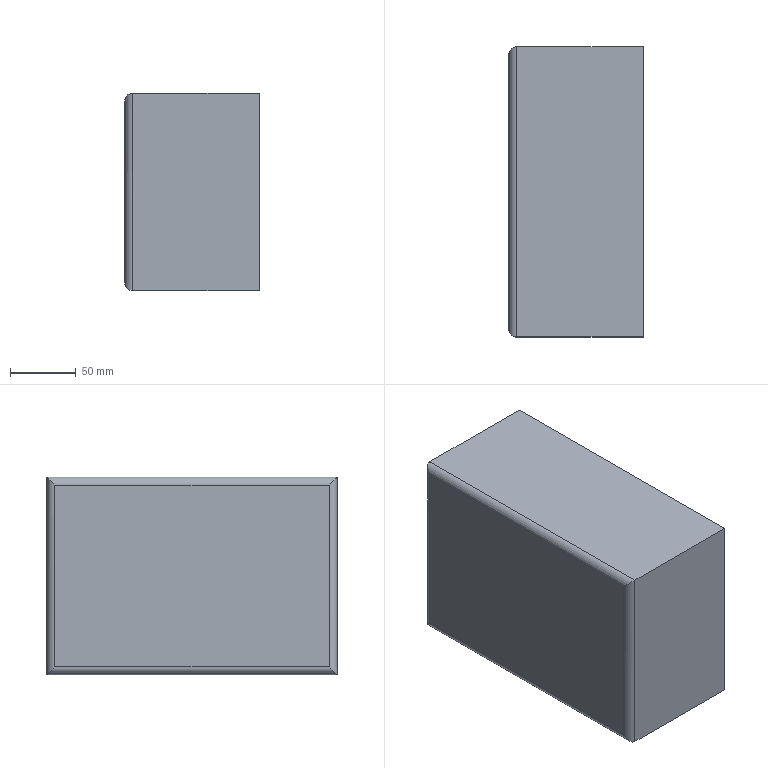Part | NX | 1 solid | 10 faces | box 102 x 220.092 x 150 mm | volume 3361772 mm3 | plane 6 | cylinder 4 | commonest cylinder face diameters 12 x4
STEP:
#1=CARTESIAN_POINT('',(-151.326,-99.951,581.553));
#2=VERTEX_POINT('',#1);
#3=CARTESIAN_POINT('',(-55.326,-99.951,581.553));
#4=VERTEX_POINT('',#3);
#5=CARTESIAN_POINT('',(-157.326,-99.951,581.553));
#6=DIRECTION('',(1.,0.,0.));
#7=VECTOR('',#6,1.);
#8=LINE('',#5,#7);
#9=EDGE_CURVE('',#2,#4,#8,.T.);
#10=ORIENTED_EDGE('',*,*,#9,.F.);
#11=CARTESIAN_POINT('',(-151.326,120.141,581.553));
#12=VERTEX_POINT('',#11);
#13=CARTESIAN_POINT('',(-151.326,120.141,581.553));
#14=DIRECTION('',(0.,1.,0.));
#15=VECTOR('',#14,1.);
#16=LINE('',#13,#15);
#17=EDGE_CURVE('',#2,#12,#16,.T.);
#18=ORIENTED_EDGE('',*,*,#17,.T.);
#19=CARTESIAN_POINT('',(-55.326,120.141,581.553));
#20=VERTEX_POINT('',#19);
#21=CARTESIAN_POINT('',(-157.326,120.141,581.553));
#22=DIRECTION('',(1.,0.,0.));
#23=VECTOR('',#22,1.);
#24=LINE('',#21,#23);
#25=EDGE_CURVE('',#12,#20,#24,.T.);
#26=ORIENTED_EDGE('',*,*,#25,.T.);
#27=CARTESIAN_POINT('',(-55.326,120.141,581.553));
#28=DIRECTION('',(0.,-1.,0.));
#29=VECTOR('',#28,1.);
#30=LINE('',#27,#29);
#31=EDGE_CURVE('',#20,#4,#30,.T.);
#32=ORIENTED_EDGE('',*,*,#31,.T.);
#33=EDGE_LOOP('',(#10,#18,#26,#32));
#34=FACE_OUTER_BOUND('',#33,.T.);
#35=CARTESIAN_POINT('',(-157.326,120.141,581.553));
#36=DIRECTION('',(0.,0.,1.));
#37=DIRECTION('',(1.,0.,0.));
#38=AXIS2_PLACEMENT_3D('',#35,#36,#37);
#39=PLANE('',#38);
#40=ADVANCED_FACE('',(#34),#39,.F.);
#41=CARTESIAN_POINT('',(-151.326,-99.951,731.553));
#42=VERTEX_POINT('',#41);
#43=CARTESIAN_POINT('',(-55.326,-99.951,731.553));
#44=VERTEX_POINT('',#43);
#45=CARTESIAN_POINT('',(-157.326,-99.951,731.553));
#46=DIRECTION('',(1.,0.,0.));
#47=VECTOR('',#46,1.);
#48=LINE('',#45,#47);
#49=EDGE_CURVE('',#42,#44,#48,.T.);
#50=ORIENTED_EDGE('',*,*,#49,.F.);
#51=CARTESIAN_POINT('',(-151.326,-99.951,581.553));
#52=DIRECTION('',(0.,0.,-1.));
#53=VECTOR('',#52,1.);
#54=LINE('',#51,#53);
#55=EDGE_CURVE('',#42,#2,#54,.T.);
#56=ORIENTED_EDGE('',*,*,#55,.T.);
#57=ORIENTED_EDGE('',*,*,#9,.T.);
#58=CARTESIAN_POINT('',(-55.326,-99.951,581.553));
#59=DIRECTION('',(0.,0.,1.));
#60=VECTOR('',#59,1.);
#61=LINE('',#58,#60);
#62=EDGE_CURVE('',#4,#44,#61,.T.);
#63=ORIENTED_EDGE('',*,*,#62,.T.);
#64=EDGE_LOOP('',(#50,#56,#57,#63));
#65=FACE_OUTER_BOUND('',#64,.T.);
#66=CARTESIAN_POINT('',(-157.326,-99.951,581.553));
#67=DIRECTION('',(0.,1.,0.));
#68=DIRECTION('',(0.,0.,1.));
#69=AXIS2_PLACEMENT_3D('',#66,#67,#68);
#70=PLANE('',#69);
#71=ADVANCED_FACE('',(#65),#70,.F.);
#72=CARTESIAN_POINT('',(-151.326,120.141,731.553));
#73=VERTEX_POINT('',#72);
#74=CARTESIAN_POINT('',(-55.326,120.141,731.553));
#75=VERTEX_POINT('',#74);
#76=CARTESIAN_POINT('',(-157.326,120.141,731.553));
#77=DIRECTION('',(1.,0.,0.));
#78=VECTOR('',#77,1.);
#79=LINE('',#76,#78);
#80=EDGE_CURVE('',#73,#75,#79,.T.);
#81=ORIENTED_EDGE('',*,*,#80,.F.);
#82=CARTESIAN_POINT('',(-151.326,-99.951,731.553));
#83=DIRECTION('',(0.,-1.,0.));
#84=VECTOR('',#83,1.);
#85=LINE('',#82,#84);
#86=EDGE_CURVE('',#73,#42,#85,.T.);
#87=ORIENTED_EDGE('',*,*,#86,.T.);
#88=ORIENTED_EDGE('',*,*,#49,.T.);
#89=CARTESIAN_POINT('',(-55.326,120.141,731.553));
#90=DIRECTION('',(0.,1.,0.));
#91=VECTOR('',#90,1.);
#92=LINE('',#89,#91);
#93=EDGE_CURVE('',#44,#75,#92,.T.);
#94=ORIENTED_EDGE('',*,*,#93,.T.);
#95=EDGE_LOOP('',(#81,#87,#88,#94));
#96=FACE_OUTER_BOUND('',#95,.T.);
#97=CARTESIAN_POINT('',(-157.326,120.141,731.553));
#98=DIRECTION('',(0.,0.,-1.));
#99=DIRECTION('',(-1.,0.,0.));
#100=AXIS2_PLACEMENT_3D('',#97,#98,#99);
#101=PLANE('',#100);
#102=ADVANCED_FACE('',(#96),#101,.F.);
#103=ORIENTED_EDGE('',*,*,#25,.F.);
#104=CARTESIAN_POINT('',(-151.326,120.141,731.553));
#105=DIRECTION('',(0.,0.,1.));
#106=VECTOR('',#105,1.);
#107=LINE('',#104,#106);
#108=EDGE_CURVE('',#12,#73,#107,.T.);
#109=ORIENTED_EDGE('',*,*,#108,.T.);
#110=ORIENTED_EDGE('',*,*,#80,.T.);
#111=CARTESIAN_POINT('',(-55.326,120.141,581.553));
#112=DIRECTION('',(0.,0.,-1.));
#113=VECTOR('',#112,1.);
#114=LINE('',#111,#113);
#115=EDGE_CURVE('',#75,#20,#114,.T.);
#116=ORIENTED_EDGE('',*,*,#115,.T.);
#117=EDGE_LOOP('',(#103,#109,#110,#116));
#118=FACE_OUTER_BOUND('',#117,.T.);
#119=CARTESIAN_POINT('',(-157.326,120.141,581.553));
#120=DIRECTION('',(0.,-1.,0.));
#121=DIRECTION('',(0.,0.,-1.));
#122=AXIS2_PLACEMENT_3D('',#119,#120,#121);
#123=PLANE('',#122);
#124=ADVANCED_FACE('',(#118),#123,.F.);
#125=CARTESIAN_POINT('',(-157.326,-93.951,725.553));
#126=VERTEX_POINT('',#125);
#127=CARTESIAN_POINT('',(-157.326,114.141,725.553));
#128=VERTEX_POINT('',#127);
#129=CARTESIAN_POINT('',(-157.326,120.141,725.553));
#130=DIRECTION('',(0.,1.,0.));
#131=VECTOR('',#130,1.);
#132=LINE('',#129,#131);
#133=EDGE_CURVE('',#126,#128,#132,.T.);
#134=ORIENTED_EDGE('',*,*,#133,.T.);
#135=CARTESIAN_POINT('',(-157.326,114.141,587.553));
#136=VERTEX_POINT('',#135);
#137=CARTESIAN_POINT('',(-157.326,114.141,581.553));
#138=DIRECTION('',(0.,0.,-1.));
#139=VECTOR('',#138,1.);
#140=LINE('',#137,#139);
#141=EDGE_CURVE('',#128,#136,#140,.T.);
#142=ORIENTED_EDGE('',*,*,#141,.T.);
#143=CARTESIAN_POINT('',(-157.326,-93.951,587.553));
#144=VERTEX_POINT('',#143);
#145=CARTESIAN_POINT('',(-157.326,-99.951,587.553));
#146=DIRECTION('',(0.,-1.,0.));
#147=VECTOR('',#146,1.);
#148=LINE('',#145,#147);
#149=EDGE_CURVE('',#136,#144,#148,.T.);
#150=ORIENTED_EDGE('',*,*,#149,.T.);
#151=CARTESIAN_POINT('',(-157.326,-93.951,731.553));
#152=DIRECTION('',(0.,0.,1.));
#153=VECTOR('',#152,1.);
#154=LINE('',#151,#153);
#155=EDGE_CURVE('',#144,#126,#154,.T.);
#156=ORIENTED_EDGE('',*,*,#155,.T.);
#157=EDGE_LOOP('',(#134,#142,#150,#156));
#158=FACE_OUTER_BOUND('',#157,.T.);
#159=CARTESIAN_POINT('',(-157.326,-99.951,581.553));
#160=DIRECTION('',(-1.,0.,0.));
#161=DIRECTION('',(0.,0.,1.));
#162=AXIS2_PLACEMENT_3D('',#159,#160,#161);
#163=PLANE('',#162);
#164=ADVANCED_FACE('',(#158),#163,.T.);
#165=ORIENTED_EDGE('',*,*,#31,.F.);
#166=ORIENTED_EDGE('',*,*,#115,.F.);
#167=ORIENTED_EDGE('',*,*,#93,.F.);
#168=ORIENTED_EDGE('',*,*,#62,.F.);
#169=EDGE_LOOP('',(#165,#166,#167,#168));
#170=FACE_OUTER_BOUND('',#169,.T.);
#171=CARTESIAN_POINT('',(-55.326,-99.951,581.553));
#172=DIRECTION('',(-1.,0.,0.));
#173=DIRECTION('',(0.,0.,1.));
#174=AXIS2_PLACEMENT_3D('',#171,#172,#173);
#175=PLANE('',#174);
#176=ADVANCED_FACE('',(#170),#175,.F.);
#177=CARTESIAN_POINT('',(-151.326,-99.951,581.553));
#178=CARTESIAN_POINT('',(-154.841,-99.951,581.553));
#179=CARTESIAN_POINT('',(-157.326,-97.465,584.039));
#180=CARTESIAN_POINT('',(-157.326,-93.951,587.553));
#181=(BOUNDED_CURVE()B_SPLINE_CURVE(3,(#177,#178,#179,#180),.UNSPECIFIED.,.F.,.F.)B_SPLINE_CURVE_WITH_KNOTS((4,4),(0.,1.),.UNSPECIFIED.)CURVE()GEOMETRIC_REPRESENTATION_ITEM()RATIONAL_B_SPLINE_CURVE((1.,0.8047,0.8047,1.))REPRESENTATION_ITEM(''));
#182=EDGE_CURVE('',#2,#144,#181,.T.);
#183=ORIENTED_EDGE('',*,*,#182,.F.);
#184=ORIENTED_EDGE('',*,*,#55,.F.);
#185=CARTESIAN_POINT('',(-157.326,-93.951,725.553));
#186=CARTESIAN_POINT('',(-157.326,-97.465,729.068));
#187=CARTESIAN_POINT('',(-154.841,-99.951,731.553));
#188=CARTESIAN_POINT('',(-151.326,-99.951,731.553));
#189=(BOUNDED_CURVE()B_SPLINE_CURVE(3,(#185,#186,#187,#188),.UNSPECIFIED.,.F.,.F.)B_SPLINE_CURVE_WITH_KNOTS((4,4),(0.,1.),.UNSPECIFIED.)CURVE()GEOMETRIC_REPRESENTATION_ITEM()RATIONAL_B_SPLINE_CURVE((1.,0.8047,0.8047,1.))REPRESENTATION_ITEM(''));
#190=EDGE_CURVE('',#126,#42,#189,.T.);
#191=ORIENTED_EDGE('',*,*,#190,.F.);
#192=ORIENTED_EDGE('',*,*,#155,.F.);
#193=EDGE_LOOP('',(#183,#184,#191,#192));
#194=FACE_OUTER_BOUND('',#193,.T.);
#195=CARTESIAN_POINT('',(-151.326,-93.951,581.553));
#196=DIRECTION('',(0.,0.,-1.));
#197=DIRECTION('',(-1.,0.,0.));
#198=AXIS2_PLACEMENT_3D('',#195,#196,#197);
#199=CYLINDRICAL_SURFACE('',#198,6.);
#200=ADVANCED_FACE('',(#194),#199,.T.);
#201=ORIENTED_EDGE('',*,*,#190,.T.);
#202=ORIENTED_EDGE('',*,*,#86,.F.);
#203=CARTESIAN_POINT('',(-157.326,114.141,725.553));
#204=CARTESIAN_POINT('',(-157.326,117.656,729.068));
#205=CARTESIAN_POINT('',(-154.841,120.141,731.553));
#206=CARTESIAN_POINT('',(-151.326,120.141,731.553));
#207=(BOUNDED_CURVE()B_SPLINE_CURVE(3,(#203,#204,#205,#206),.UNSPECIFIED.,.F.,.F.)B_SPLINE_CURVE_WITH_KNOTS((4,4),(0.,1.),.UNSPECIFIED.)CURVE()GEOMETRIC_REPRESENTATION_ITEM()RATIONAL_B_SPLINE_CURVE((1.,0.8047,0.8047,1.))REPRESENTATION_ITEM(''));
#208=EDGE_CURVE('',#128,#73,#207,.T.);
#209=ORIENTED_EDGE('',*,*,#208,.F.);
#210=ORIENTED_EDGE('',*,*,#133,.F.);
#211=EDGE_LOOP('',(#201,#202,#209,#210));
#212=FACE_OUTER_BOUND('',#211,.T.);
#213=CARTESIAN_POINT('',(-151.326,-99.951,725.553));
#214=DIRECTION('',(0.,-1.,0.));
#215=DIRECTION('',(0.,0.,-1.));
#216=AXIS2_PLACEMENT_3D('',#213,#214,#215);
#217=CYLINDRICAL_SURFACE('',#216,6.);
#218=ADVANCED_FACE('',(#212),#217,.T.);
#219=ORIENTED_EDGE('',*,*,#182,.T.);
#220=ORIENTED_EDGE('',*,*,#149,.F.);
#221=CARTESIAN_POINT('',(-151.326,120.141,581.553));
#222=CARTESIAN_POINT('',(-154.841,120.141,581.553));
#223=CARTESIAN_POINT('',(-157.326,117.656,584.039));
#224=CARTESIAN_POINT('',(-157.326,114.141,587.553));
#225=(BOUNDED_CURVE()B_SPLINE_CURVE(3,(#221,#222,#223,#224),.UNSPECIFIED.,.F.,.F.)B_SPLINE_CURVE_WITH_KNOTS((4,4),(0.,1.),.UNSPECIFIED.)CURVE()GEOMETRIC_REPRESENTATION_ITEM()RATIONAL_B_SPLINE_CURVE((1.,0.8047,0.8047,1.))REPRESENTATION_ITEM(''));
#226=EDGE_CURVE('',#12,#136,#225,.T.);
#227=ORIENTED_EDGE('',*,*,#226,.F.);
#228=ORIENTED_EDGE('',*,*,#17,.F.);
#229=EDGE_LOOP('',(#219,#220,#227,#228));
#230=FACE_OUTER_BOUND('',#229,.T.);
#231=CARTESIAN_POINT('',(-151.326,-99.951,587.553));
#232=DIRECTION('',(0.,1.,0.));
#233=DIRECTION('',(0.,0.,1.));
#234=AXIS2_PLACEMENT_3D('',#231,#232,#233);
#235=CYLINDRICAL_SURFACE('',#234,6.);
#236=ADVANCED_FACE('',(#230),#235,.T.);
#237=ORIENTED_EDGE('',*,*,#208,.T.);
#238=ORIENTED_EDGE('',*,*,#108,.F.);
#239=ORIENTED_EDGE('',*,*,#226,.T.);
#240=ORIENTED_EDGE('',*,*,#141,.F.);
#241=EDGE_LOOP('',(#237,#238,#239,#240));
#242=FACE_OUTER_BOUND('',#241,.T.);
#243=CARTESIAN_POINT('',(-151.326,114.141,581.553));
#244=DIRECTION('',(0.,0.,1.));
#245=DIRECTION('',(1.,0.,0.));
#246=AXIS2_PLACEMENT_3D('',#243,#244,#245);
#247=CYLINDRICAL_SURFACE('',#246,6.);
#248=ADVANCED_FACE('',(#242),#247,.T.);
#249=CLOSED_SHELL('',(#40,#71,#102,#124,#164,#176,#200,#218,#236,#248));
#250=MANIFOLD_SOLID_BREP('',#249);
#251=(LENGTH_UNIT()NAMED_UNIT(*)SI_UNIT(.MILLI.,.METRE.));
#252=UNCERTAINTY_MEASURE_WITH_UNIT(LENGTH_MEASURE(0.00002),#251,'','');
#253=(NAMED_UNIT(*)PLANE_ANGLE_UNIT()SI_UNIT($,.RADIAN.));
#254=PLANE_ANGLE_MEASURE_WITH_UNIT(PLANE_ANGLE_MEASURE(0.01745),#253);
#255=DIMENSIONAL_EXPONENTS(0.,0.,0.,0.,0.,0.,0.);
#256=(CONVERSION_BASED_UNIT('DEGREE',#254)NAMED_UNIT(#255)PLANE_ANGLE_UNIT());
#257=(NAMED_UNIT(*)SI_UNIT($,.STERADIAN.)SOLID_ANGLE_UNIT());
#258=(GEOMETRIC_REPRESENTATION_CONTEXT(3)GLOBAL_UNCERTAINTY_ASSIGNED_CONTEXT((#252))GLOBAL_UNIT_ASSIGNED_CONTEXT((#251,#256,#257))REPRESENTATION_CONTEXT('',''));
#259=ADVANCED_BREP_SHAPE_REPRESENTATION('',(#250),#258);